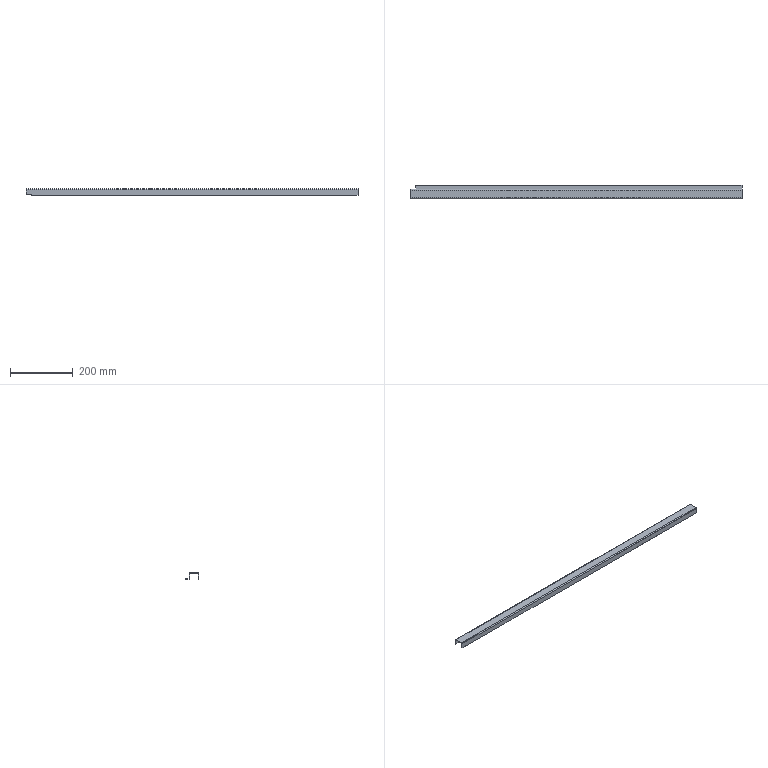Part | SolidWorks | features BaseBody 1 | 1 solid | 36 faces | box 1059 x 43 x 20 mm | volume 161287 mm3 | plane 30 | cylinder 6 | commonest cylinder face diameters 2 x3 6 x3
STEP:
#1=CARTESIAN_POINT('',(-529.5,-13.,-18.));
#2=VERTEX_POINT('',#1);
#3=CARTESIAN_POINT('',(-512.5,-13.,-18.));
#4=VERTEX_POINT('',#3);
#5=CARTESIAN_POINT('',(0.,-13.,-18.));
#6=DIRECTION('',(1.,0.,0.));
#7=VECTOR('',#6,1000.);
#8=LINE('',#5,#7);
#9=EDGE_CURVE('',#2,#4,#8,.T.);
#10=ORIENTED_EDGE('',*,*,#9,.T.);
#11=CARTESIAN_POINT('',(-512.5,-15.,-18.));
#12=VERTEX_POINT('',#11);
#13=CARTESIAN_POINT('',(-512.5,-15.,-18.));
#14=DIRECTION('',(0.,1.,0.));
#15=VECTOR('',#14,1000.);
#16=LINE('',#13,#15);
#17=EDGE_CURVE('',#12,#4,#16,.T.);
#18=ORIENTED_EDGE('',*,*,#17,.F.);
#19=CARTESIAN_POINT('',(-529.5,-15.,-18.));
#20=VERTEX_POINT('',#19);
#21=CARTESIAN_POINT('',(-529.5,-15.,-18.));
#22=DIRECTION('',(1.,0.,0.));
#23=VECTOR('',#22,1000.);
#24=LINE('',#21,#23);
#25=EDGE_CURVE('',#20,#12,#24,.T.);
#26=ORIENTED_EDGE('',*,*,#25,.F.);
#27=CARTESIAN_POINT('',(-529.5,-15.,-18.));
#28=DIRECTION('',(0.,1.,0.));
#29=VECTOR('',#28,1000.);
#30=LINE('',#27,#29);
#31=EDGE_CURVE('',#20,#2,#30,.T.);
#32=ORIENTED_EDGE('',*,*,#31,.T.);
#33=EDGE_LOOP('',(#10,#18,#26,#32));
#34=FACE_OUTER_BOUND('',#33,.T.);
#35=CARTESIAN_POINT('',(-529.5,-15.,-18.));
#36=DIRECTION('',(0.,0.,1.));
#37=DIRECTION('',(0.,-1.,0.));
#38=AXIS2_PLACEMENT_3D('',#35,#36,#37);
#39=PLANE('',#38);
#40=ADVANCED_FACE('',(#34),#39,.F.);
#41=CARTESIAN_POINT('',(-512.5,-13.,-20.));
#42=VERTEX_POINT('',#41);
#43=CARTESIAN_POINT('',(-512.5,-13.,0.));
#44=DIRECTION('',(0.,0.,-1.));
#45=VECTOR('',#44,1000.);
#46=LINE('',#43,#45);
#47=EDGE_CURVE('',#4,#42,#46,.T.);
#48=ORIENTED_EDGE('',*,*,#47,.T.);
#49=CARTESIAN_POINT('',(-512.5,-15.,-20.));
#50=VERTEX_POINT('',#49);
#51=CARTESIAN_POINT('',(-512.5,-15.,-20.));
#52=DIRECTION('',(0.,1.,0.));
#53=VECTOR('',#52,1000.);
#54=LINE('',#51,#53);
#55=EDGE_CURVE('',#50,#42,#54,.T.);
#56=ORIENTED_EDGE('',*,*,#55,.F.);
#57=CARTESIAN_POINT('',(-512.5,-15.,-20.));
#58=DIRECTION('',(0.,0.,-1.));
#59=VECTOR('',#58,1000.);
#60=LINE('',#57,#59);
#61=EDGE_CURVE('',#12,#50,#60,.T.);
#62=ORIENTED_EDGE('',*,*,#61,.F.);
#63=ORIENTED_EDGE('',*,*,#17,.T.);
#64=EDGE_LOOP('',(#48,#56,#62,#63));
#65=FACE_OUTER_BOUND('',#64,.T.);
#66=CARTESIAN_POINT('',(-512.5,-15.,-20.));
#67=DIRECTION('',(1.,0.,0.));
#68=DIRECTION('',(0.,1.,0.));
#69=AXIS2_PLACEMENT_3D('',#66,#67,#68);
#70=PLANE('',#69);
#71=ADVANCED_FACE('',(#65),#70,.F.);
#72=CARTESIAN_POINT('',(-529.5,13.,-18.));
#73=VERTEX_POINT('',#72);
#74=CARTESIAN_POINT('',(-529.5,15.,-18.));
#75=VERTEX_POINT('',#74);
#76=CARTESIAN_POINT('',(-529.5,-15.,-18.));
#77=DIRECTION('',(0.,1.,0.));
#78=VECTOR('',#77,1000.);
#79=LINE('',#76,#78);
#80=EDGE_CURVE('',#73,#75,#79,.T.);
#81=ORIENTED_EDGE('',*,*,#80,.T.);
#82=CARTESIAN_POINT('',(-512.5,15.,-18.));
#83=VERTEX_POINT('',#82);
#84=CARTESIAN_POINT('',(-529.5,15.,-18.));
#85=DIRECTION('',(1.,0.,0.));
#86=VECTOR('',#85,1000.);
#87=LINE('',#84,#86);
#88=EDGE_CURVE('',#75,#83,#87,.T.);
#89=ORIENTED_EDGE('',*,*,#88,.T.);
#90=CARTESIAN_POINT('',(-512.5,13.,-18.));
#91=VERTEX_POINT('',#90);
#92=CARTESIAN_POINT('',(-512.5,15.,-18.));
#93=DIRECTION('',(0.,-1.,0.));
#94=VECTOR('',#93,1000.);
#95=LINE('',#92,#94);
#96=EDGE_CURVE('',#83,#91,#95,.T.);
#97=ORIENTED_EDGE('',*,*,#96,.T.);
#98=CARTESIAN_POINT('',(0.,13.,-18.));
#99=DIRECTION('',(1.,0.,0.));
#100=VECTOR('',#99,1000.);
#101=LINE('',#98,#100);
#102=EDGE_CURVE('',#73,#91,#101,.T.);
#103=ORIENTED_EDGE('',*,*,#102,.F.);
#104=EDGE_LOOP('',(#81,#89,#97,#103));
#105=FACE_OUTER_BOUND('',#104,.T.);
#106=CARTESIAN_POINT('',(-529.5,-15.,-18.));
#107=DIRECTION('',(0.,0.,1.));
#108=DIRECTION('',(0.,-1.,0.));
#109=AXIS2_PLACEMENT_3D('',#106,#107,#108);
#110=PLANE('',#109);
#111=ADVANCED_FACE('',(#105),#110,.F.);
#112=CARTESIAN_POINT('',(-511.5,28.,-18.));
#113=VERTEX_POINT('',#112);
#114=CARTESIAN_POINT('',(529.5,28.,-18.));
#115=VERTEX_POINT('',#114);
#116=CARTESIAN_POINT('',(529.5,28.,-18.));
#117=DIRECTION('',(1.,0.,0.));
#118=VECTOR('',#117,1000.);
#119=LINE('',#116,#118);
#120=EDGE_CURVE('',#113,#115,#119,.T.);
#121=ORIENTED_EDGE('',*,*,#120,.T.);
#122=CARTESIAN_POINT('',(529.5,28.,-20.));
#123=VERTEX_POINT('',#122);
#124=CARTESIAN_POINT('',(529.5,28.,-20.));
#125=DIRECTION('',(0.,0.,1.));
#126=VECTOR('',#125,1000.);
#127=LINE('',#124,#126);
#128=EDGE_CURVE('',#123,#115,#127,.T.);
#129=ORIENTED_EDGE('',*,*,#128,.F.);
#130=CARTESIAN_POINT('',(-511.5,28.,-20.));
#131=VERTEX_POINT('',#130);
#132=CARTESIAN_POINT('',(0.,28.,-20.));
#133=DIRECTION('',(1.,0.,0.));
#134=VECTOR('',#133,1000.);
#135=LINE('',#132,#134);
#136=EDGE_CURVE('',#131,#123,#135,.T.);
#137=ORIENTED_EDGE('',*,*,#136,.F.);
#138=CARTESIAN_POINT('',(-511.5,28.,-20.));
#139=DIRECTION('',(0.,0.,1.));
#140=VECTOR('',#139,1000.);
#141=LINE('',#138,#140);
#142=EDGE_CURVE('',#131,#113,#141,.T.);
#143=ORIENTED_EDGE('',*,*,#142,.T.);
#144=EDGE_LOOP('',(#121,#129,#137,#143));
#145=FACE_OUTER_BOUND('',#144,.T.);
#146=CARTESIAN_POINT('',(529.5,28.,-20.));
#147=DIRECTION('',(0.,-1.,0.));
#148=DIRECTION('',(-1.,0.,0.));
#149=AXIS2_PLACEMENT_3D('',#146,#147,#148);
#150=PLANE('',#149);
#151=ADVANCED_FACE('',(#145),#150,.F.);
#152=CARTESIAN_POINT('',(-511.5,16.,-18.));
#153=VERTEX_POINT('',#152);
#154=CARTESIAN_POINT('',(-511.5,15.,-18.));
#155=DIRECTION('',(0.,1.,0.));
#156=VECTOR('',#155,1000.);
#157=LINE('',#154,#156);
#158=EDGE_CURVE('',#153,#113,#157,.T.);
#159=ORIENTED_EDGE('',*,*,#158,.F.);
#160=CARTESIAN_POINT('',(529.5,16.,-18.));
#161=VERTEX_POINT('',#160);
#162=CARTESIAN_POINT('',(529.5,16.,-18.));
#163=DIRECTION('',(-1.,0.,0.));
#164=VECTOR('',#163,1000.);
#165=LINE('',#162,#164);
#166=EDGE_CURVE('',#161,#153,#165,.T.);
#167=ORIENTED_EDGE('',*,*,#166,.F.);
#168=CARTESIAN_POINT('',(529.5,15.,-18.));
#169=DIRECTION('',(0.,-1.,0.));
#170=VECTOR('',#169,1000.);
#171=LINE('',#168,#170);
#172=EDGE_CURVE('',#115,#161,#171,.T.);
#173=ORIENTED_EDGE('',*,*,#172,.F.);
#174=ORIENTED_EDGE('',*,*,#120,.F.);
#175=EDGE_LOOP('',(#159,#167,#173,#174));
#176=FACE_OUTER_BOUND('',#175,.T.);
#177=CARTESIAN_POINT('',(0.,0.,-18.));
#178=DIRECTION('',(0.,0.,1.));
#179=DIRECTION('',(1.,0.,0.));
#180=AXIS2_PLACEMENT_3D('',#177,#178,#179);
#181=PLANE('',#180);
#182=ADVANCED_FACE('',(#176),#181,.T.);
#183=CARTESIAN_POINT('',(-511.5,16.,-20.));
#184=VERTEX_POINT('',#183);
#185=CARTESIAN_POINT('',(529.5,16.,-20.));
#186=VERTEX_POINT('',#185);
#187=CARTESIAN_POINT('',(529.5,16.,-20.));
#188=DIRECTION('',(1.,0.,0.));
#189=VECTOR('',#188,1000.);
#190=LINE('',#187,#189);
#191=EDGE_CURVE('',#184,#186,#190,.T.);
#192=ORIENTED_EDGE('',*,*,#191,.F.);
#193=CARTESIAN_POINT('',(-511.5,0.,-20.));
#194=DIRECTION('',(0.,1.,0.));
#195=VECTOR('',#194,1000.);
#196=LINE('',#193,#195);
#197=EDGE_CURVE('',#184,#131,#196,.T.);
#198=ORIENTED_EDGE('',*,*,#197,.T.);
#199=ORIENTED_EDGE('',*,*,#136,.T.);
#200=CARTESIAN_POINT('',(529.5,0.,-20.));
#201=DIRECTION('',(0.,-1.,0.));
#202=VECTOR('',#201,1000.);
#203=LINE('',#200,#202);
#204=EDGE_CURVE('',#123,#186,#203,.T.);
#205=ORIENTED_EDGE('',*,*,#204,.T.);
#206=EDGE_LOOP('',(#192,#198,#199,#205));
#207=FACE_OUTER_BOUND('',#206,.T.);
#208=CARTESIAN_POINT('',(0.,0.,-20.));
#209=DIRECTION('',(0.,0.,1.));
#210=DIRECTION('',(1.,0.,0.));
#211=AXIS2_PLACEMENT_3D('',#208,#209,#210);
#212=PLANE('',#211);
#213=ADVANCED_FACE('',(#207),#212,.F.);
#214=CARTESIAN_POINT('',(-511.5,16.,-18.));
#215=DIRECTION('',(0.,0.,-1.));
#216=VECTOR('',#215,1000.);
#217=LINE('',#214,#216);
#218=EDGE_CURVE('',#153,#184,#217,.T.);
#219=ORIENTED_EDGE('',*,*,#218,.F.);
#220=ORIENTED_EDGE('',*,*,#158,.T.);
#221=ORIENTED_EDGE('',*,*,#142,.F.);
#222=ORIENTED_EDGE('',*,*,#197,.F.);
#223=EDGE_LOOP('',(#219,#220,#221,#222));
#224=FACE_OUTER_BOUND('',#223,.T.);
#225=CARTESIAN_POINT('',(-511.5,15.,-20.));
#226=DIRECTION('',(1.,0.,0.));
#227=DIRECTION('',(0.,1.,0.));
#228=AXIS2_PLACEMENT_3D('',#225,#226,#227);
#229=PLANE('',#228);
#230=ADVANCED_FACE('',(#224),#229,.F.);
#231=CARTESIAN_POINT('',(529.5,16.,-20.));
#232=DIRECTION('',(0.,0.,-1.));
#233=VECTOR('',#232,1000.);
#234=LINE('',#231,#233);
#235=EDGE_CURVE('',#161,#186,#234,.T.);
#236=ORIENTED_EDGE('',*,*,#235,.T.);
#237=ORIENTED_EDGE('',*,*,#204,.F.);
#238=ORIENTED_EDGE('',*,*,#128,.T.);
#239=ORIENTED_EDGE('',*,*,#172,.T.);
#240=EDGE_LOOP('',(#236,#237,#238,#239));
#241=FACE_OUTER_BOUND('',#240,.T.);
#242=CARTESIAN_POINT('',(529.5,15.,-20.));
#243=DIRECTION('',(-1.,0.,0.));
#244=DIRECTION('',(0.,0.,1.));
#245=AXIS2_PLACEMENT_3D('',#242,#243,#244);
#246=PLANE('',#245);
#247=ADVANCED_FACE('',(#241),#246,.F.);
#248=CARTESIAN_POINT('',(-511.5,15.,-17.));
#249=VERTEX_POINT('',#248);
#250=CARTESIAN_POINT('',(529.5,15.,-17.));
#251=VERTEX_POINT('',#250);
#252=CARTESIAN_POINT('',(-511.5,15.,-17.));
#253=DIRECTION('',(1.,0.,0.));
#254=VECTOR('',#253,1000.);
#255=LINE('',#252,#254);
#256=EDGE_CURVE('',#249,#251,#255,.T.);
#257=ORIENTED_EDGE('',*,*,#256,.T.);
#258=CARTESIAN_POINT('',(529.5,16.,-17.));
#259=DIRECTION('',(1.,0.,0.));
#260=DIRECTION('',(0.,0.,1.));
#261=AXIS2_PLACEMENT_3D('',#258,#259,#260);
#262=CIRCLE('',#261,1.);
#263=EDGE_CURVE('',#251,#161,#262,.T.);
#264=ORIENTED_EDGE('',*,*,#263,.T.);
#265=ORIENTED_EDGE('',*,*,#166,.T.);
#266=CARTESIAN_POINT('',(-511.5,16.,-17.));
#267=DIRECTION('',(-1.,0.,0.));
#268=DIRECTION('',(0.,0.,1.));
#269=AXIS2_PLACEMENT_3D('',#266,#267,#268);
#270=CIRCLE('',#269,1.);
#271=EDGE_CURVE('',#153,#249,#270,.T.);
#272=ORIENTED_EDGE('',*,*,#271,.T.);
#273=EDGE_LOOP('',(#257,#264,#265,#272));
#274=FACE_OUTER_BOUND('',#273,.T.);
#275=CARTESIAN_POINT('',(-511.5,16.,-17.));
#276=DIRECTION('',(-1.,0.,0.));
#277=DIRECTION('',(0.,0.,-1.));
#278=AXIS2_PLACEMENT_3D('',#275,#276,#277);
#279=CYLINDRICAL_SURFACE('',#278,1.);
#280=ADVANCED_FACE('',(#274),#279,.F.);
#281=CARTESIAN_POINT('',(-511.5,13.,-17.));
#282=VERTEX_POINT('',#281);
#283=CARTESIAN_POINT('',(529.5,13.,-17.));
#284=VERTEX_POINT('',#283);
#285=CARTESIAN_POINT('',(-511.5,13.,-17.));
#286=DIRECTION('',(1.,0.,0.));
#287=VECTOR('',#286,1000.);
#288=LINE('',#285,#287);
#289=EDGE_CURVE('',#282,#284,#288,.T.);
#290=ORIENTED_EDGE('',*,*,#289,.F.);
#291=CARTESIAN_POINT('',(-511.5,16.,-17.));
#292=DIRECTION('',(-1.,0.,0.));
#293=DIRECTION('',(0.,0.,1.));
#294=AXIS2_PLACEMENT_3D('',#291,#292,#293);
#295=CIRCLE('',#294,3.);
#296=EDGE_CURVE('',#184,#282,#295,.T.);
#297=ORIENTED_EDGE('',*,*,#296,.F.);
#298=ORIENTED_EDGE('',*,*,#191,.T.);
#299=CARTESIAN_POINT('',(529.5,16.,-17.));
#300=DIRECTION('',(1.,0.,0.));
#301=DIRECTION('',(0.,0.,1.));
#302=AXIS2_PLACEMENT_3D('',#299,#300,#301);
#303=CIRCLE('',#302,3.);
#304=EDGE_CURVE('',#284,#186,#303,.T.);
#305=ORIENTED_EDGE('',*,*,#304,.F.);
#306=EDGE_LOOP('',(#290,#297,#298,#305));
#307=FACE_OUTER_BOUND('',#306,.T.);
#308=CARTESIAN_POINT('',(-511.5,16.,-17.));
#309=DIRECTION('',(-1.,0.,0.));
#310=DIRECTION('',(0.,0.,-1.));
#311=AXIS2_PLACEMENT_3D('',#308,#309,#310);
#312=CYLINDRICAL_SURFACE('',#311,3.);
#313=ADVANCED_FACE('',(#307),#312,.T.);
#314=ORIENTED_EDGE('',*,*,#271,.F.);
#315=ORIENTED_EDGE('',*,*,#218,.T.);
#316=ORIENTED_EDGE('',*,*,#296,.T.);
#317=CARTESIAN_POINT('',(-511.5,15.,-17.));
#318=DIRECTION('',(0.,-1.,0.));
#319=VECTOR('',#318,1000.);
#320=LINE('',#317,#319);
#321=EDGE_CURVE('',#249,#282,#320,.T.);
#322=ORIENTED_EDGE('',*,*,#321,.F.);
#323=EDGE_LOOP('',(#314,#315,#316,#322));
#324=FACE_OUTER_BOUND('',#323,.T.);
#325=CARTESIAN_POINT('',(-511.5,16.,-17.));
#326=DIRECTION('',(1.,0.,0.));
#327=DIRECTION('',(0.,1.,0.));
#328=AXIS2_PLACEMENT_3D('',#325,#326,#327);
#329=PLANE('',#328);
#330=ADVANCED_FACE('',(#324),#329,.F.);
#331=ORIENTED_EDGE('',*,*,#235,.F.);
#332=ORIENTED_EDGE('',*,*,#263,.F.);
#333=CARTESIAN_POINT('',(529.5,15.,-17.));
#334=DIRECTION('',(0.,-1.,0.));
#335=VECTOR('',#334,1000.);
#336=LINE('',#333,#335);
#337=EDGE_CURVE('',#251,#284,#336,.T.);
#338=ORIENTED_EDGE('',*,*,#337,.T.);
#339=ORIENTED_EDGE('',*,*,#304,.T.);
#340=EDGE_LOOP('',(#331,#332,#338,#339));
#341=FACE_OUTER_BOUND('',#340,.T.);
#342=CARTESIAN_POINT('',(529.5,16.,-17.));
#343=DIRECTION('',(1.,0.,0.));
#344=DIRECTION('',(0.,1.,0.));
#345=AXIS2_PLACEMENT_3D('',#342,#343,#344);
#346=PLANE('',#345);
#347=ADVANCED_FACE('',(#341),#346,.T.);
#348=ORIENTED_EDGE('',*,*,#96,.F.);
#349=CARTESIAN_POINT('',(-512.5,15.,-16.));
#350=VERTEX_POINT('',#349);
#351=CARTESIAN_POINT('',(-512.5,15.,-20.));
#352=DIRECTION('',(0.,0.,1.));
#353=VECTOR('',#352,1000.);
#354=LINE('',#351,#353);
#355=EDGE_CURVE('',#83,#350,#354,.T.);
#356=ORIENTED_EDGE('',*,*,#355,.T.);
#357=CARTESIAN_POINT('',(-512.5,13.,-16.));
#358=VERTEX_POINT('',#357);
#359=CARTESIAN_POINT('',(-512.5,15.,-16.));
#360=DIRECTION('',(0.,-1.,0.));
#361=VECTOR('',#360,1000.);
#362=LINE('',#359,#361);
#363=EDGE_CURVE('',#350,#358,#362,.T.);
#364=ORIENTED_EDGE('',*,*,#363,.T.);
#365=CARTESIAN_POINT('',(-512.5,13.,0.));
#366=DIRECTION('',(0.,0.,-1.));
#367=VECTOR('',#366,1000.);
#368=LINE('',#365,#367);
#369=EDGE_CURVE('',#358,#91,#368,.T.);
#370=ORIENTED_EDGE('',*,*,#369,.T.);
#371=EDGE_LOOP('',(#348,#356,#364,#370));
#372=FACE_OUTER_BOUND('',#371,.T.);
#373=CARTESIAN_POINT('',(-512.5,15.,-20.));
#374=DIRECTION('',(1.,0.,0.));
#375=DIRECTION('',(0.,0.,1.));
#376=AXIS2_PLACEMENT_3D('',#373,#374,#375);
#377=PLANE('',#376);
#378=ADVANCED_FACE('',(#372),#377,.T.);
#379=ORIENTED_EDGE('',*,*,#321,.T.);
#380=CARTESIAN_POINT('',(-511.5,13.,-16.));
#381=VERTEX_POINT('',#380);
#382=CARTESIAN_POINT('',(-511.5,13.,0.));
#383=DIRECTION('',(0.,0.,1.));
#384=VECTOR('',#383,1000.);
#385=LINE('',#382,#384);
#386=EDGE_CURVE('',#282,#381,#385,.T.);
#387=ORIENTED_EDGE('',*,*,#386,.T.);
#388=CARTESIAN_POINT('',(-511.5,15.,-16.));
#389=VERTEX_POINT('',#388);
#390=CARTESIAN_POINT('',(-511.5,15.,-16.));
#391=DIRECTION('',(0.,-1.,0.));
#392=VECTOR('',#391,1000.);
#393=LINE('',#390,#392);
#394=EDGE_CURVE('',#389,#381,#393,.T.);
#395=ORIENTED_EDGE('',*,*,#394,.F.);
#396=CARTESIAN_POINT('',(-511.5,15.,-16.));
#397=DIRECTION('',(0.,0.,-1.));
#398=VECTOR('',#397,1000.);
#399=LINE('',#396,#398);
#400=EDGE_CURVE('',#389,#249,#399,.T.);
#401=ORIENTED_EDGE('',*,*,#400,.T.);
#402=EDGE_LOOP('',(#379,#387,#395,#401));
#403=FACE_OUTER_BOUND('',#402,.T.);
#404=CARTESIAN_POINT('',(-511.5,15.,-16.));
#405=DIRECTION('',(-1.,0.,0.));
#406=DIRECTION('',(0.,0.,1.));
#407=AXIS2_PLACEMENT_3D('',#404,#405,#406);
#408=PLANE('',#407);
#409=ADVANCED_FACE('',(#403),#408,.T.);
#410=ORIENTED_EDGE('',*,*,#394,.T.);
#411=CARTESIAN_POINT('',(0.,13.,-16.));
#412=DIRECTION('',(-1.,0.,0.));
#413=VECTOR('',#412,1000.);
#414=LINE('',#411,#413);
#415=EDGE_CURVE('',#381,#358,#414,.T.);
#416=ORIENTED_EDGE('',*,*,#415,.T.);
#417=ORIENTED_EDGE('',*,*,#363,.F.);
#418=CARTESIAN_POINT('',(-512.5,15.,-16.));
#419=DIRECTION('',(1.,0.,0.));
#420=VECTOR('',#419,1000.);
#421=LINE('',#418,#420);
#422=EDGE_CURVE('',#350,#389,#421,.T.);
#423=ORIENTED_EDGE('',*,*,#422,.T.);
#424=EDGE_LOOP('',(#410,#416,#417,#423));
#425=FACE_OUTER_BOUND('',#424,.T.);
#426=CARTESIAN_POINT('',(-512.5,15.,-16.));
#427=DIRECTION('',(0.,0.,-1.));
#428=DIRECTION('',(-1.,0.,0.));
#429=AXIS2_PLACEMENT_3D('',#426,#427,#428);
#430=PLANE('',#429);
#431=ADVANCED_FACE('',(#425),#430,.T.);
#432=ORIENTED_EDGE('',*,*,#55,.T.);
#433=CARTESIAN_POINT('',(529.5,-13.,-20.));
#434=VERTEX_POINT('',#433);
#435=CARTESIAN_POINT('',(0.,-13.,-20.));
#436=DIRECTION('',(-1.,0.,0.));
#437=VECTOR('',#436,1000.);
#438=LINE('',#435,#437);
#439=EDGE_CURVE('',#434,#42,#438,.T.);
#440=ORIENTED_EDGE('',*,*,#439,.F.);
#441=CARTESIAN_POINT('',(529.5,-15.,-20.));
#442=VERTEX_POINT('',#441);
#443=CARTESIAN_POINT('',(529.5,-15.,-20.));
#444=DIRECTION('',(0.,1.,0.));
#445=VECTOR('',#444,1000.);
#446=LINE('',#443,#445);
#447=EDGE_CURVE('',#442,#434,#446,.T.);
#448=ORIENTED_EDGE('',*,*,#447,.F.);
#449=CARTESIAN_POINT('',(529.5,-15.,-20.));
#450=DIRECTION('',(-1.,0.,0.));
#451=VECTOR('',#450,1000.);
#452=LINE('',#449,#451);
#453=EDGE_CURVE('',#442,#50,#452,.T.);
#454=ORIENTED_EDGE('',*,*,#453,.T.);
#455=EDGE_LOOP('',(#432,#440,#448,#454));
#456=FACE_OUTER_BOUND('',#455,.T.);
#457=CARTESIAN_POINT('',(529.5,-15.,-20.));
#458=DIRECTION('',(0.,0.,-1.));
#459=DIRECTION('',(0.,-1.,0.));
#460=AXIS2_PLACEMENT_3D('',#457,#458,#459);
#461=PLANE('',#460);
#462=ADVANCED_FACE('',(#456),#461,.T.);
#463=ORIENTED_EDGE('',*,*,#47,.F.);
#464=ORIENTED_EDGE('',*,*,#9,.F.);
#465=CARTESIAN_POINT('',(-529.5,-13.,-3.));
#466=VERTEX_POINT('',#465);
#467=CARTESIAN_POINT('',(-529.5,-13.,0.));
#468=DIRECTION('',(0.,0.,1.));
#469=VECTOR('',#468,1000.);
#470=LINE('',#467,#469);
#471=EDGE_CURVE('',#2,#466,#470,.T.);
#472=ORIENTED_EDGE('',*,*,#471,.T.);
#473=CARTESIAN_POINT('',(529.5,-13.,-3.));
#474=VERTEX_POINT('',#473);
#475=CARTESIAN_POINT('',(529.5,-13.,-3.));
#476=DIRECTION('',(-1.,0.,0.));
#477=VECTOR('',#476,1000.);
#478=LINE('',#475,#477);
#479=EDGE_CURVE('',#474,#466,#478,.T.);
#480=ORIENTED_EDGE('',*,*,#479,.F.);
#481=CARTESIAN_POINT('',(529.5,-13.,0.));
#482=DIRECTION('',(0.,0.,-1.));
#483=VECTOR('',#482,1000.);
#484=LINE('',#481,#483);
#485=EDGE_CURVE('',#474,#434,#484,.T.);
#486=ORIENTED_EDGE('',*,*,#485,.T.);
#487=ORIENTED_EDGE('',*,*,#439,.T.);
#488=EDGE_LOOP('',(#463,#464,#472,#480,#486,#487));
#489=FACE_OUTER_BOUND('',#488,.T.);
#490=CARTESIAN_POINT('',(0.,-13.,0.));
#491=DIRECTION('',(0.,1.,0.));
#492=DIRECTION('',(0.,0.,-1.));
#493=AXIS2_PLACEMENT_3D('',#490,#491,#492);
#494=PLANE('',#493);
#495=ADVANCED_FACE('',(#489),#494,.T.);
#496=ORIENTED_EDGE('',*,*,#25,.T.);
#497=ORIENTED_EDGE('',*,*,#61,.T.);
#498=ORIENTED_EDGE('',*,*,#453,.F.);
#499=CARTESIAN_POINT('',(529.5,-15.,-3.));
#500=VERTEX_POINT('',#499);
#501=CARTESIAN_POINT('',(529.5,-15.,-2.));
#502=DIRECTION('',(0.,0.,-1.));
#503=VECTOR('',#502,1000.);
#504=LINE('',#501,#503);
#505=EDGE_CURVE('',#500,#442,#504,.T.);
#506=ORIENTED_EDGE('',*,*,#505,.F.);
#507=CARTESIAN_POINT('',(-529.5,-15.,-3.));
#508=VERTEX_POINT('',#507);
#509=CARTESIAN_POINT('',(529.5,-15.,-3.));
#510=DIRECTION('',(1.,0.,0.));
#511=VECTOR('',#510,1000.);
#512=LINE('',#509,#511);
#513=EDGE_CURVE('',#508,#500,#512,.T.);
#514=ORIENTED_EDGE('',*,*,#513,.F.);
#515=CARTESIAN_POINT('',(-529.5,-15.,-20.));
#516=DIRECTION('',(0.,0.,1.));
#517=VECTOR('',#516,1000.);
#518=LINE('',#515,#517);
#519=EDGE_CURVE('',#20,#508,#518,.T.);
#520=ORIENTED_EDGE('',*,*,#519,.F.);
#521=EDGE_LOOP('',(#496,#497,#498,#506,#514,#520));
#522=FACE_OUTER_BOUND('',#521,.T.);
#523=CARTESIAN_POINT('',(0.,-15.,0.));
#524=DIRECTION('',(0.,1.,0.));
#525=DIRECTION('',(0.,0.,-1.));
#526=AXIS2_PLACEMENT_3D('',#523,#524,#525);
#527=PLANE('',#526);
#528=ADVANCED_FACE('',(#522),#527,.F.);
#529=ORIENTED_EDGE('',*,*,#31,.F.);
#530=ORIENTED_EDGE('',*,*,#519,.T.);
#531=CARTESIAN_POINT('',(-529.5,-13.,-3.));
#532=DIRECTION('',(0.,-1.,0.));
#533=VECTOR('',#532,1000.);
#534=LINE('',#531,#533);
#535=EDGE_CURVE('',#466,#508,#534,.T.);
#536=ORIENTED_EDGE('',*,*,#535,.F.);
#537=ORIENTED_EDGE('',*,*,#471,.F.);
#538=EDGE_LOOP('',(#529,#530,#536,#537));
#539=FACE_OUTER_BOUND('',#538,.T.);
#540=CARTESIAN_POINT('',(-529.5,-15.,-20.));
#541=DIRECTION('',(-1.,0.,0.));
#542=DIRECTION('',(0.,0.,1.));
#543=AXIS2_PLACEMENT_3D('',#540,#541,#542);
#544=PLANE('',#543);
#545=ADVANCED_FACE('',(#539),#544,.T.);
#546=ORIENTED_EDGE('',*,*,#485,.F.);
#547=CARTESIAN_POINT('',(529.5,-15.,-3.));
#548=DIRECTION('',(0.,-1.,0.));
#549=VECTOR('',#548,1000.);
#550=LINE('',#547,#549);
#551=EDGE_CURVE('',#474,#500,#550,.T.);
#552=ORIENTED_EDGE('',*,*,#551,.T.);
#553=ORIENTED_EDGE('',*,*,#505,.T.);
#554=ORIENTED_EDGE('',*,*,#447,.T.);
#555=EDGE_LOOP('',(#546,#552,#553,#554));
#556=FACE_OUTER_BOUND('',#555,.T.);
#557=CARTESIAN_POINT('',(529.5,-15.,-2.));
#558=DIRECTION('',(1.,0.,0.));
#559=DIRECTION('',(0.,1.,0.));
#560=AXIS2_PLACEMENT_3D('',#557,#558,#559);
#561=PLANE('',#560);
#562=ADVANCED_FACE('',(#556),#561,.T.);
#563=CARTESIAN_POINT('',(-529.5,-12.,-2.));
#564=VERTEX_POINT('',#563);
#565=CARTESIAN_POINT('',(529.5,-12.,-2.));
#566=VERTEX_POINT('',#565);
#567=CARTESIAN_POINT('',(-529.5,-12.,-2.));
#568=DIRECTION('',(1.,0.,0.));
#569=VECTOR('',#568,1000.);
#570=LINE('',#567,#569);
#571=EDGE_CURVE('',#564,#566,#570,.T.);
#572=ORIENTED_EDGE('',*,*,#571,.T.);
#573=CARTESIAN_POINT('',(529.5,-12.,-3.));
#574=DIRECTION('',(1.,0.,0.));
#575=DIRECTION('',(0.,0.,1.));
#576=AXIS2_PLACEMENT_3D('',#573,#574,#575);
#577=CIRCLE('',#576,1.);
#578=EDGE_CURVE('',#566,#474,#577,.T.);
#579=ORIENTED_EDGE('',*,*,#578,.T.);
#580=ORIENTED_EDGE('',*,*,#479,.T.);
#581=CARTESIAN_POINT('',(-529.5,-12.,-3.));
#582=DIRECTION('',(-1.,0.,0.));
#583=DIRECTION('',(0.,0.,1.));
#584=AXIS2_PLACEMENT_3D('',#581,#582,#583);
#585=CIRCLE('',#584,1.);
#586=EDGE_CURVE('',#466,#564,#585,.T.);
#587=ORIENTED_EDGE('',*,*,#586,.T.);
#588=EDGE_LOOP('',(#572,#579,#580,#587));
#589=FACE_OUTER_BOUND('',#588,.T.);
#590=CARTESIAN_POINT('',(-529.5,-12.,-3.));
#591=DIRECTION('',(-1.,0.,0.));
#592=DIRECTION('',(0.,-1.,0.));
#593=AXIS2_PLACEMENT_3D('',#590,#591,#592);
#594=CYLINDRICAL_SURFACE('',#593,1.);
#595=ADVANCED_FACE('',(#589),#594,.F.);
#596=CARTESIAN_POINT('',(-529.5,-12.,0.));
#597=VERTEX_POINT('',#596);
#598=CARTESIAN_POINT('',(529.5,-12.,0.));
#599=VERTEX_POINT('',#598);
#600=CARTESIAN_POINT('',(-529.5,-12.,0.));
#601=DIRECTION('',(1.,0.,0.));
#602=VECTOR('',#601,1000.);
#603=LINE('',#600,#602);
#604=EDGE_CURVE('',#597,#599,#603,.T.);
#605=ORIENTED_EDGE('',*,*,#604,.F.);
#606=CARTESIAN_POINT('',(-529.5,-12.,-3.));
#607=DIRECTION('',(-1.,0.,0.));
#608=DIRECTION('',(0.,0.,1.));
#609=AXIS2_PLACEMENT_3D('',#606,#607,#608);
#610=CIRCLE('',#609,3.);
#611=EDGE_CURVE('',#508,#597,#610,.T.);
#612=ORIENTED_EDGE('',*,*,#611,.F.);
#613=ORIENTED_EDGE('',*,*,#513,.T.);
#614=CARTESIAN_POINT('',(529.5,-12.,-3.));
#615=DIRECTION('',(1.,0.,0.));
#616=DIRECTION('',(0.,0.,1.));
#617=AXIS2_PLACEMENT_3D('',#614,#615,#616);
#618=CIRCLE('',#617,3.);
#619=EDGE_CURVE('',#599,#500,#618,.T.);
#620=ORIENTED_EDGE('',*,*,#619,.F.);
#621=EDGE_LOOP('',(#605,#612,#613,#620));
#622=FACE_OUTER_BOUND('',#621,.T.);
#623=CARTESIAN_POINT('',(-529.5,-12.,-3.));
#624=DIRECTION('',(-1.,0.,0.));
#625=DIRECTION('',(0.,-1.,0.));
#626=AXIS2_PLACEMENT_3D('',#623,#624,#625);
#627=CYLINDRICAL_SURFACE('',#626,3.);
#628=ADVANCED_FACE('',(#622),#627,.T.);
#629=ORIENTED_EDGE('',*,*,#586,.F.);
#630=ORIENTED_EDGE('',*,*,#535,.T.);
#631=ORIENTED_EDGE('',*,*,#611,.T.);
#632=CARTESIAN_POINT('',(-529.5,-12.,-2.));
#633=DIRECTION('',(0.,0.,1.));
#634=VECTOR('',#633,1000.);
#635=LINE('',#632,#634);
#636=EDGE_CURVE('',#564,#597,#635,.T.);
#637=ORIENTED_EDGE('',*,*,#636,.F.);
#638=EDGE_LOOP('',(#629,#630,#631,#637));
#639=FACE_OUTER_BOUND('',#638,.T.);
#640=CARTESIAN_POINT('',(-529.5,-12.,-3.));
#641=DIRECTION('',(1.,0.,0.));
#642=DIRECTION('',(0.,1.,0.));
#643=AXIS2_PLACEMENT_3D('',#640,#641,#642);
#644=PLANE('',#643);
#645=ADVANCED_FACE('',(#639),#644,.F.);
#646=ORIENTED_EDGE('',*,*,#551,.F.);
#647=ORIENTED_EDGE('',*,*,#578,.F.);
#648=CARTESIAN_POINT('',(529.5,-12.,-2.));
#649=DIRECTION('',(0.,0.,1.));
#650=VECTOR('',#649,1000.);
#651=LINE('',#648,#650);
#652=EDGE_CURVE('',#566,#599,#651,.T.);
#653=ORIENTED_EDGE('',*,*,#652,.T.);
#654=ORIENTED_EDGE('',*,*,#619,.T.);
#655=EDGE_LOOP('',(#646,#647,#653,#654));
#656=FACE_OUTER_BOUND('',#655,.T.);
#657=CARTESIAN_POINT('',(529.5,-12.,-3.));
#658=DIRECTION('',(1.,0.,0.));
#659=DIRECTION('',(0.,1.,0.));
#660=AXIS2_PLACEMENT_3D('',#657,#658,#659);
#661=PLANE('',#660);
#662=ADVANCED_FACE('',(#656),#661,.T.);
#663=ORIENTED_EDGE('',*,*,#80,.F.);
#664=CARTESIAN_POINT('',(-529.5,13.,-3.));
#665=VERTEX_POINT('',#664);
#666=CARTESIAN_POINT('',(-529.5,13.,0.));
#667=DIRECTION('',(0.,0.,-1.));
#668=VECTOR('',#667,1000.);
#669=LINE('',#666,#668);
#670=EDGE_CURVE('',#665,#73,#669,.T.);
#671=ORIENTED_EDGE('',*,*,#670,.F.);
#672=CARTESIAN_POINT('',(-529.5,15.,-3.));
#673=VERTEX_POINT('',#672);
#674=CARTESIAN_POINT('',(-529.5,15.,-3.));
#675=DIRECTION('',(0.,1.,0.));
#676=VECTOR('',#675,1000.);
#677=LINE('',#674,#676);
#678=EDGE_CURVE('',#665,#673,#677,.T.);
#679=ORIENTED_EDGE('',*,*,#678,.T.);
#680=CARTESIAN_POINT('',(-529.5,15.,-20.));
#681=DIRECTION('',(0.,0.,-1.));
#682=VECTOR('',#681,1000.);
#683=LINE('',#680,#682);
#684=EDGE_CURVE('',#673,#75,#683,.T.);
#685=ORIENTED_EDGE('',*,*,#684,.T.);
#686=EDGE_LOOP('',(#663,#671,#679,#685));
#687=FACE_OUTER_BOUND('',#686,.T.);
#688=CARTESIAN_POINT('',(-529.5,15.,-20.));
#689=DIRECTION('',(-1.,0.,0.));
#690=DIRECTION('',(0.,0.,1.));
#691=AXIS2_PLACEMENT_3D('',#688,#689,#690);
#692=PLANE('',#691);
#693=ADVANCED_FACE('',(#687),#692,.T.);
#694=ORIENTED_EDGE('',*,*,#337,.F.);
#695=CARTESIAN_POINT('',(529.5,15.,-3.));
#696=VERTEX_POINT('',#695);
#697=CARTESIAN_POINT('',(529.5,15.,-2.));
#698=DIRECTION('',(0.,0.,1.));
#699=VECTOR('',#698,1000.);
#700=LINE('',#697,#699);
#701=EDGE_CURVE('',#251,#696,#700,.T.);
#702=ORIENTED_EDGE('',*,*,#701,.T.);
#703=CARTESIAN_POINT('',(529.5,13.,-3.));
#704=VERTEX_POINT('',#703);
#705=CARTESIAN_POINT('',(529.5,13.,-3.));
#706=DIRECTION('',(0.,1.,0.));
#707=VECTOR('',#706,1000.);
#708=LINE('',#705,#707);
#709=EDGE_CURVE('',#704,#696,#708,.T.);
#710=ORIENTED_EDGE('',*,*,#709,.F.);
#711=CARTESIAN_POINT('',(529.5,13.,0.));
#712=DIRECTION('',(0.,0.,1.));
#713=VECTOR('',#712,1000.);
#714=LINE('',#711,#713);
#715=EDGE_CURVE('',#284,#704,#714,.T.);
#716=ORIENTED_EDGE('',*,*,#715,.F.);
#717=EDGE_LOOP('',(#694,#702,#710,#716));
#718=FACE_OUTER_BOUND('',#717,.T.);
#719=CARTESIAN_POINT('',(529.5,15.,-2.));
#720=DIRECTION('',(1.,0.,0.));
#721=DIRECTION('',(0.,1.,0.));
#722=AXIS2_PLACEMENT_3D('',#719,#720,#721);
#723=PLANE('',#722);
#724=ADVANCED_FACE('',(#718),#723,.T.);
#725=CARTESIAN_POINT('',(529.5,12.,-2.));
#726=VERTEX_POINT('',#725);
#727=CARTESIAN_POINT('',(-529.5,12.,-2.));
#728=VERTEX_POINT('',#727);
#729=CARTESIAN_POINT('',(529.5,12.,-2.));
#730=DIRECTION('',(-1.,0.,0.));
#731=VECTOR('',#730,1000.);
#732=LINE('',#729,#731);
#733=EDGE_CURVE('',#726,#728,#732,.T.);
#734=ORIENTED_EDGE('',*,*,#733,.T.);
#735=CARTESIAN_POINT('',(-529.5,12.,-3.));
#736=DIRECTION('',(-1.,0.,0.));
#737=DIRECTION('',(0.,0.,-1.));
#738=AXIS2_PLACEMENT_3D('',#735,#736,#737);
#739=CIRCLE('',#738,1.);
#740=EDGE_CURVE('',#728,#665,#739,.T.);
#741=ORIENTED_EDGE('',*,*,#740,.T.);
#742=CARTESIAN_POINT('',(-529.5,13.,-3.));
#743=DIRECTION('',(1.,0.,0.));
#744=VECTOR('',#743,1000.);
#745=LINE('',#742,#744);
#746=EDGE_CURVE('',#665,#704,#745,.T.);
#747=ORIENTED_EDGE('',*,*,#746,.T.);
#748=CARTESIAN_POINT('',(529.5,12.,-3.));
#749=DIRECTION('',(1.,0.,0.));
#750=DIRECTION('',(0.,0.,-1.));
#751=AXIS2_PLACEMENT_3D('',#748,#749,#750);
#752=CIRCLE('',#751,1.);
#753=EDGE_CURVE('',#704,#726,#752,.T.);
#754=ORIENTED_EDGE('',*,*,#753,.T.);
#755=EDGE_LOOP('',(#734,#741,#747,#754));
#756=FACE_OUTER_BOUND('',#755,.T.);
#757=CARTESIAN_POINT('',(529.5,12.,-3.));
#758=DIRECTION('',(1.,0.,0.));
#759=DIRECTION('',(0.,1.,0.));
#760=AXIS2_PLACEMENT_3D('',#757,#758,#759);
#761=CYLINDRICAL_SURFACE('',#760,1.);
#762=ADVANCED_FACE('',(#756),#761,.F.);
#763=CARTESIAN_POINT('',(529.5,12.,0.));
#764=VERTEX_POINT('',#763);
#765=CARTESIAN_POINT('',(-529.5,12.,0.));
#766=VERTEX_POINT('',#765);
#767=CARTESIAN_POINT('',(529.5,12.,0.));
#768=DIRECTION('',(-1.,0.,0.));
#769=VECTOR('',#768,1000.);
#770=LINE('',#767,#769);
#771=EDGE_CURVE('',#764,#766,#770,.T.);
#772=ORIENTED_EDGE('',*,*,#771,.F.);
#773=CARTESIAN_POINT('',(529.5,12.,-3.));
#774=DIRECTION('',(1.,0.,0.));
#775=DIRECTION('',(0.,0.,-1.));
#776=AXIS2_PLACEMENT_3D('',#773,#774,#775);
#777=CIRCLE('',#776,3.);
#778=EDGE_CURVE('',#696,#764,#777,.T.);
#779=ORIENTED_EDGE('',*,*,#778,.F.);
#780=CARTESIAN_POINT('',(0.,15.,-3.));
#781=DIRECTION('',(1.,0.,0.));
#782=VECTOR('',#781,1000.);
#783=LINE('',#780,#782);
#784=EDGE_CURVE('',#673,#696,#783,.T.);
#785=ORIENTED_EDGE('',*,*,#784,.F.);
#786=CARTESIAN_POINT('',(-529.5,12.,-3.));
#787=DIRECTION('',(-1.,0.,0.));
#788=DIRECTION('',(0.,0.,-1.));
#789=AXIS2_PLACEMENT_3D('',#786,#787,#788);
#790=CIRCLE('',#789,3.);
#791=EDGE_CURVE('',#766,#673,#790,.T.);
#792=ORIENTED_EDGE('',*,*,#791,.F.);
#793=EDGE_LOOP('',(#772,#779,#785,#792));
#794=FACE_OUTER_BOUND('',#793,.T.);
#795=CARTESIAN_POINT('',(529.5,12.,-3.));
#796=DIRECTION('',(1.,0.,0.));
#797=DIRECTION('',(0.,1.,0.));
#798=AXIS2_PLACEMENT_3D('',#795,#796,#797);
#799=CYLINDRICAL_SURFACE('',#798,3.);
#800=ADVANCED_FACE('',(#794),#799,.T.);
#801=ORIENTED_EDGE('',*,*,#753,.F.);
#802=ORIENTED_EDGE('',*,*,#709,.T.);
#803=ORIENTED_EDGE('',*,*,#778,.T.);
#804=CARTESIAN_POINT('',(529.5,12.,-2.));
#805=DIRECTION('',(0.,0.,1.));
#806=VECTOR('',#805,1000.);
#807=LINE('',#804,#806);
#808=EDGE_CURVE('',#726,#764,#807,.T.);
#809=ORIENTED_EDGE('',*,*,#808,.F.);
#810=EDGE_LOOP('',(#801,#802,#803,#809));
#811=FACE_OUTER_BOUND('',#810,.T.);
#812=CARTESIAN_POINT('',(529.5,12.,-3.));
#813=DIRECTION('',(-1.,0.,0.));
#814=DIRECTION('',(0.,0.,1.));
#815=AXIS2_PLACEMENT_3D('',#812,#813,#814);
#816=PLANE('',#815);
#817=ADVANCED_FACE('',(#811),#816,.F.);
#818=ORIENTED_EDGE('',*,*,#678,.F.);
#819=ORIENTED_EDGE('',*,*,#740,.F.);
#820=CARTESIAN_POINT('',(-529.5,12.,-2.));
#821=DIRECTION('',(0.,0.,1.));
#822=VECTOR('',#821,1000.);
#823=LINE('',#820,#822);
#824=EDGE_CURVE('',#728,#766,#823,.T.);
#825=ORIENTED_EDGE('',*,*,#824,.T.);
#826=ORIENTED_EDGE('',*,*,#791,.T.);
#827=EDGE_LOOP('',(#818,#819,#825,#826));
#828=FACE_OUTER_BOUND('',#827,.T.);
#829=CARTESIAN_POINT('',(-529.5,12.,-3.));
#830=DIRECTION('',(-1.,0.,0.));
#831=DIRECTION('',(0.,0.,1.));
#832=AXIS2_PLACEMENT_3D('',#829,#830,#831);
#833=PLANE('',#832);
#834=ADVANCED_FACE('',(#828),#833,.T.);
#835=ORIENTED_EDGE('',*,*,#652,.F.);
#836=CARTESIAN_POINT('',(529.5,15.,-2.));
#837=DIRECTION('',(0.,1.,0.));
#838=VECTOR('',#837,1000.);
#839=LINE('',#836,#838);
#840=EDGE_CURVE('',#566,#726,#839,.T.);
#841=ORIENTED_EDGE('',*,*,#840,.T.);
#842=ORIENTED_EDGE('',*,*,#808,.T.);
#843=CARTESIAN_POINT('',(529.5,15.,0.));
#844=DIRECTION('',(0.,1.,0.));
#845=VECTOR('',#844,1000.);
#846=LINE('',#843,#845);
#847=EDGE_CURVE('',#599,#764,#846,.T.);
#848=ORIENTED_EDGE('',*,*,#847,.F.);
#849=EDGE_LOOP('',(#835,#841,#842,#848));
#850=FACE_OUTER_BOUND('',#849,.T.);
#851=CARTESIAN_POINT('',(529.5,15.,-2.));
#852=DIRECTION('',(1.,0.,0.));
#853=DIRECTION('',(0.,1.,0.));
#854=AXIS2_PLACEMENT_3D('',#851,#852,#853);
#855=PLANE('',#854);
#856=ADVANCED_FACE('',(#850),#855,.T.);
#857=CARTESIAN_POINT('',(-529.5,15.,-2.));
#858=DIRECTION('',(0.,-1.,0.));
#859=VECTOR('',#858,1000.);
#860=LINE('',#857,#859);
#861=EDGE_CURVE('',#728,#564,#860,.T.);
#862=ORIENTED_EDGE('',*,*,#861,.T.);
#863=ORIENTED_EDGE('',*,*,#636,.T.);
#864=CARTESIAN_POINT('',(-529.5,15.,0.));
#865=DIRECTION('',(0.,-1.,0.));
#866=VECTOR('',#865,1000.);
#867=LINE('',#864,#866);
#868=EDGE_CURVE('',#766,#597,#867,.T.);
#869=ORIENTED_EDGE('',*,*,#868,.F.);
#870=ORIENTED_EDGE('',*,*,#824,.F.);
#871=EDGE_LOOP('',(#862,#863,#869,#870));
#872=FACE_OUTER_BOUND('',#871,.T.);
#873=CARTESIAN_POINT('',(-529.5,15.,-2.));
#874=DIRECTION('',(-1.,0.,0.));
#875=DIRECTION('',(0.,0.,1.));
#876=AXIS2_PLACEMENT_3D('',#873,#874,#875);
#877=PLANE('',#876);
#878=ADVANCED_FACE('',(#872),#877,.T.);
#879=ORIENTED_EDGE('',*,*,#868,.T.);
#880=ORIENTED_EDGE('',*,*,#604,.T.);
#881=ORIENTED_EDGE('',*,*,#847,.T.);
#882=ORIENTED_EDGE('',*,*,#771,.T.);
#883=EDGE_LOOP('',(#879,#880,#881,#882));
#884=FACE_OUTER_BOUND('',#883,.T.);
#885=CARTESIAN_POINT('',(0.,0.,0.));
#886=DIRECTION('',(0.,0.,1.));
#887=DIRECTION('',(1.,0.,0.));
#888=AXIS2_PLACEMENT_3D('',#885,#886,#887);
#889=PLANE('',#888);
#890=ADVANCED_FACE('',(#884),#889,.T.);
#891=ORIENTED_EDGE('',*,*,#571,.F.);
#892=ORIENTED_EDGE('',*,*,#861,.F.);
#893=ORIENTED_EDGE('',*,*,#733,.F.);
#894=ORIENTED_EDGE('',*,*,#840,.F.);
#895=EDGE_LOOP('',(#891,#892,#893,#894));
#896=FACE_OUTER_BOUND('',#895,.T.);
#897=CARTESIAN_POINT('',(0.,0.,-2.));
#898=DIRECTION('',(0.,0.,1.));
#899=DIRECTION('',(1.,0.,0.));
#900=AXIS2_PLACEMENT_3D('',#897,#898,#899);
#901=PLANE('',#900);
#902=ADVANCED_FACE('',(#896),#901,.F.);
#903=ORIENTED_EDGE('',*,*,#670,.T.);
#904=ORIENTED_EDGE('',*,*,#102,.T.);
#905=ORIENTED_EDGE('',*,*,#369,.F.);
#906=ORIENTED_EDGE('',*,*,#415,.F.);
#907=ORIENTED_EDGE('',*,*,#386,.F.);
#908=ORIENTED_EDGE('',*,*,#289,.T.);
#909=ORIENTED_EDGE('',*,*,#715,.T.);
#910=ORIENTED_EDGE('',*,*,#746,.F.);
#911=EDGE_LOOP('',(#903,#904,#905,#906,#907,#908,#909,#910));
#912=FACE_OUTER_BOUND('',#911,.T.);
#913=CARTESIAN_POINT('',(0.,13.,0.));
#914=DIRECTION('',(0.,1.,0.));
#915=DIRECTION('',(0.,0.,-1.));
#916=AXIS2_PLACEMENT_3D('',#913,#914,#915);
#917=PLANE('',#916);
#918=ADVANCED_FACE('',(#912),#917,.F.);
#919=ORIENTED_EDGE('',*,*,#88,.F.);
#920=ORIENTED_EDGE('',*,*,#684,.F.);
#921=ORIENTED_EDGE('',*,*,#784,.T.);
#922=ORIENTED_EDGE('',*,*,#701,.F.);
#923=ORIENTED_EDGE('',*,*,#256,.F.);
#924=ORIENTED_EDGE('',*,*,#400,.F.);
#925=ORIENTED_EDGE('',*,*,#422,.F.);
#926=ORIENTED_EDGE('',*,*,#355,.F.);
#927=EDGE_LOOP('',(#919,#920,#921,#922,#923,#924,#925,#926));
#928=FACE_OUTER_BOUND('',#927,.T.);
#929=CARTESIAN_POINT('',(0.,15.,0.));
#930=DIRECTION('',(0.,1.,0.));
#931=DIRECTION('',(0.,0.,-1.));
#932=AXIS2_PLACEMENT_3D('',#929,#930,#931);
#933=PLANE('',#932);
#934=ADVANCED_FACE('',(#928),#933,.T.);
#935=CLOSED_SHELL('',(#40,#71,#111,#151,#182,#213,#230,#247,#280,#313,#330,#347,#378,#409,#431,#462,#495,#528,#545,#562,#595,#628,#645,#662,#693,#724,#762,#800,#817,#834,#856,#878,#890,#902,#918,#934));
#936=MANIFOLD_SOLID_BREP('',#935);
#937=CARTESIAN_POINT('',(0.,0.,0.));
#938=DIRECTION('',(0.,0.,1.));
#939=DIRECTION('',(1.,0.,0.));
#940=AXIS2_PLACEMENT_3D('',#937,#938,#939);
#941=(LENGTH_UNIT()NAMED_UNIT(*)SI_UNIT(.MILLI.,.METRE.));
#942=UNCERTAINTY_MEASURE_WITH_UNIT(LENGTH_MEASURE(0.00001),#941,'','');
#943=(NAMED_UNIT(*)PLANE_ANGLE_UNIT()SI_UNIT($,.RADIAN.));
#944=(NAMED_UNIT(*)SI_UNIT($,.STERADIAN.)SOLID_ANGLE_UNIT());
#945=(GEOMETRIC_REPRESENTATION_CONTEXT(3)GLOBAL_UNCERTAINTY_ASSIGNED_CONTEXT((#942))GLOBAL_UNIT_ASSIGNED_CONTEXT((#941,#943,#944))REPRESENTATION_CONTEXT('',''));
#946=ADVANCED_BREP_SHAPE_REPRESENTATION('',(#936,#940),#945);